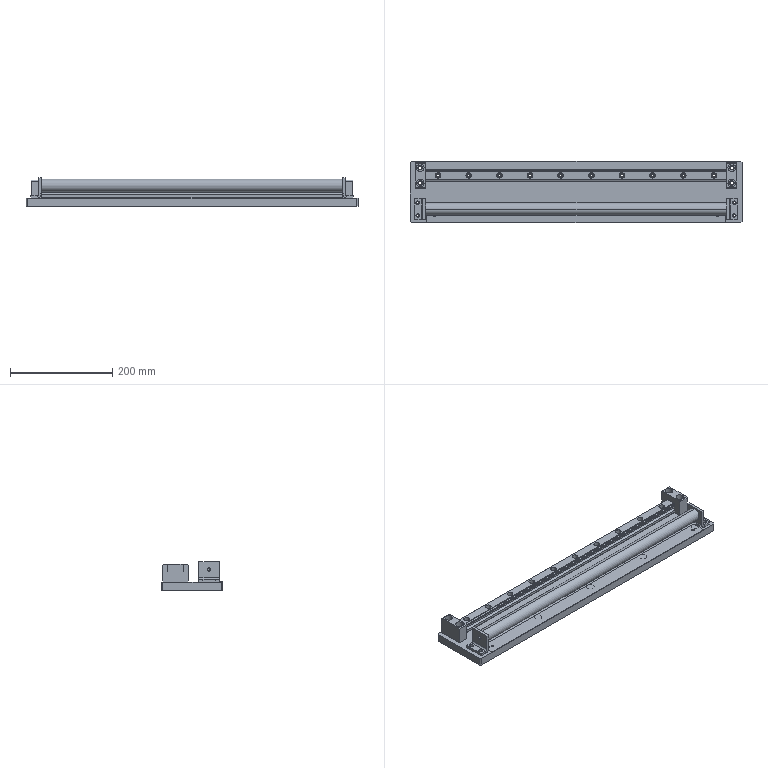Part | SolidWorks | features CompositeCurve 2 | 8 solids | 257 faces | box 650 x 120 x 55.5 mm | volume 1855069 mm3 | cylinder 148 | plane 99 | cone 10 | commonest cylinder face diameters 5 x32 7 x32 11 x20 9 x18 15 x18 6.8 x12